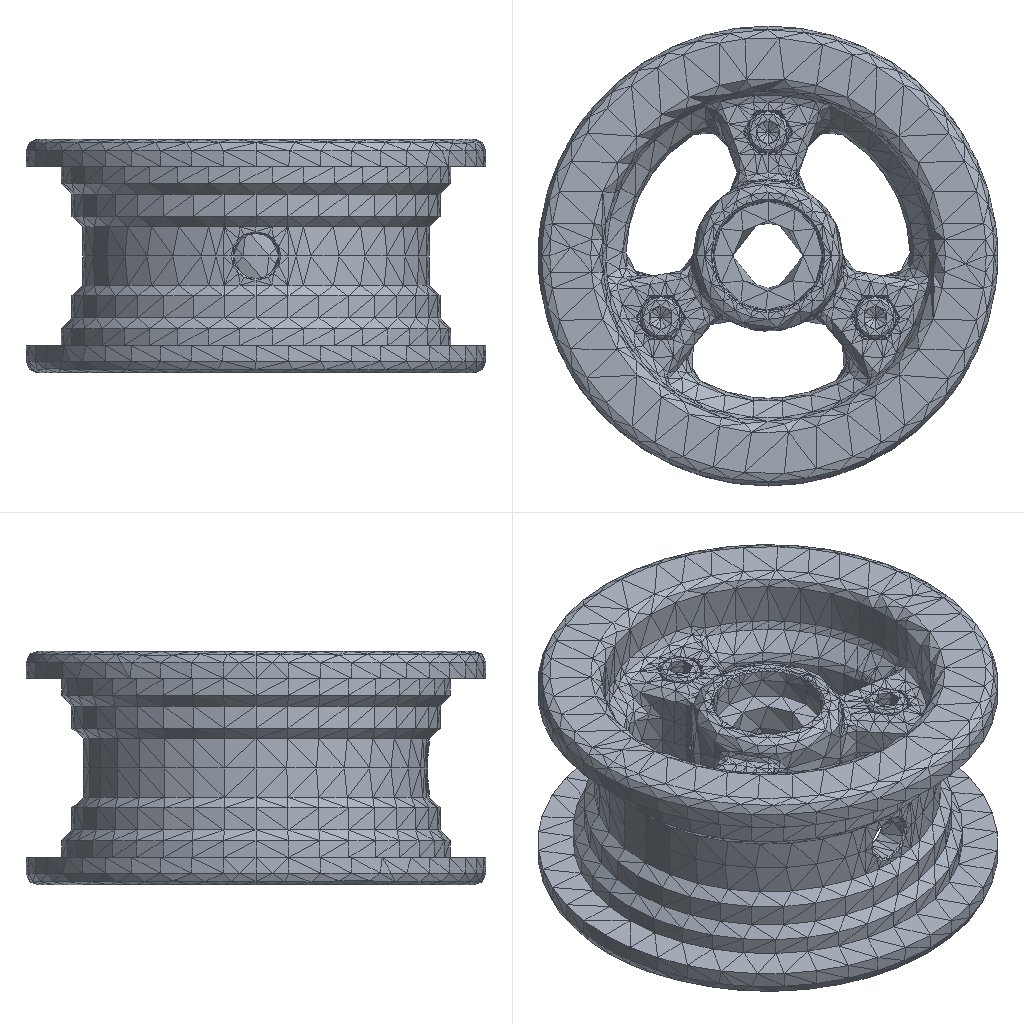Simulation study | ansys workbench
Ansys APDL input file, long lists of numbers shortened:
/batch
/config,noeldb,1     ! force off writing results to database
*get,_wallstrt,active,,time,wall
! ANSYS input file written by Workbench version 2022 R1
! File used for geometry attach:
/title,wbnew--__ (B5)
! ****** Begin Custom Load Command Snippet ******
/COM, ACT Extensions:
/COM,     LSDYNA, 2021.1
/COM,
! ****** End   Custom Load Command Snippet ******
*DIM,_wb_ProjectScratch_dir,string,248
_wb_ProjectScratch_dir(1) = ''
*DIM,_wb_SolverFiles_dir,string,248
_wb_SolverFiles_dir(1) = ''
*DIM,_wb_userfiles_dir,string,248
_wb_userfiles_dir(1) = ''
/com,--- Data in consistent NMM units. See Solving Units in the help system for more information.
/units,MPA
/nopr
/wb,file,start              !  signify a WB generated input file
/prep7
! Turn off shape checking because checks already performed inside WB mesher.
! See help system for more information.
SHPP,OFF,,NOWARN
/nolist
etcon,set             ! allow ANSYS to choose best KEYOP's for 180x elements, resets any applicable keyopt to MAPDL defaults
/com,*********** Nodes for the whole assembly ***********
nblock,3,,38121
(1i9,3e20.9e3)
        1    -7.914531287E+01    -4.780604649E+00     3.826096569E+01
! (34655 more lines like these left out)
-1
/wb,elem,start            !  set before creation of elements
/com,*********** Elements for Body 1 "Wheel Hub|Pah4" ***********
et,1,187
eblock,19,solid,,6596
(19i9)
        1        1        1        1        0        0        0        0       10        0     5341    10933    11707    12259    11913    16847    20987    16852    16849
! (13191 more lines like these left out)
-1
/com,*********** Elements for Body 2 "Wheel Hub|Pah4[2]" ***********
et,2,187
eblock,19,solid,,6596
(19i9)
        2        2        2        2        0        0        0        0       10        0    11937    23119    23893    24445    24099    29033    33173    29038    29035
! (13191 more lines like these left out)
-1
/com,*********** Elements for Body 3 "socket head cap screw_am32323_PreviewCfg|____1" ***********
et,3,187
eblock,19,solid,,671
(19i9)
        3        3        3        3        0        0        0        0       10        0     1343     2584     2701     2791     2775     2902     3548     2908     2906
! (1341 more lines like these left out)
-1
/com,*********** Elements for Body 4 "socket head cap screw_am32323_PreviewCfg|____1[2]" ***********
et,4,187
eblock,19,solid,,671
(19i9)
        4        4        4        4        0        0        0        0       10        0        1       12      129      219      203      330      976      336      334
! (1341 more lines like these left out)
-1
/com,*********** Elements for Body 5 "socket head cap screw_am32323_PreviewCfg|____1[3]" ***********
et,5,187
eblock,19,solid,,671
(19i9)
        5        5        5        5        0        0        0        0       10        0      672     1298     1415     1505     1489     1616     2262     1622     1620
! (1341 more lines like these left out)
-1
/com,*********** Elements for Body 6 "hex nut style 1_am333_PreviewCfg|____1" ***********
et,6,187
eblock,19,solid,,1109
(19i9)
        6        6        6        6        0        0        0        0       10        0     2014     4166     4227     4189     4221     5872     5956     5868     5870
! (2217 more lines like these left out)
-1
/com,*********** Elements for Body 7 "hex nut style 1_am333_PreviewCfg|____1[2]" ***********
et,7,187
eblock,19,solid,,1109
(19i9)
        7        7        7        7        0        0        0        0       10        0     3123     6308     6369     6331     6363     8014     8098     8010     8012
! (2217 more lines like these left out)
-1
/com,*********** Elements for Body 8 "hex nut style 1_am333_PreviewCfg|____1[3]" ***********
et,8,187
eblock,19,solid,,1109
(19i9)
        8        8        8        8        0        0        0        0       10        0     4232     8450     8511     8473     8505    10156    10240    10152    10154
! (2217 more lines like these left out)
-1
/wb,elem,end               !  done creating elements
/com,*********** Send User Defined Coordinate System(s) ***********
csys,0
toffst,273.15,  ! Temperature offset from absolute zero
/com,*********** Set Reference Temperature ***********
tref,22.
/wb,mat,start              !  starting to send materials
/com,*********** Send Materials ***********
Temperature = 'TEMP' ! Temperature
MP,DENS,1,7.85e-09,	! tonne mm^-3
MP,ALPX,1,1.2e-05,	! C^-1
MP,C,1,434000000,	! mm^2 s^-2 C^-1
MP,KXX,1,60.5,	! tonne mm s^-3 C^-1
MP,RSVX,1,0.00017,	! ohm mm
MP,EX,1,200000,	! tonne s^-2 mm^-1
MP,NUXY,1,0.3,
MP,MURX,1,10000,
Temperature = 'TEMP' ! Temperature
MP,DENS,2,7.85e-09,	! tonne mm^-3
MP,ALPX,2,1.2e-05,	! C^-1
MP,C,2,434000000,	! mm^2 s^-2 C^-1
MP,KXX,2,60.5,	! tonne mm s^-3 C^-1
MP,RSVX,2,0.00017,	! ohm mm
MP,EX,2,200000,	! tonne s^-2 mm^-1
MP,NUXY,2,0.3,
MP,MURX,2,10000,
Temperature = 'TEMP' ! Temperature
MP,DENS,3,7.85e-09,	! tonne mm^-3
MP,ALPX,3,1.2e-05,	! C^-1
MP,C,3,434000000,	! mm^2 s^-2 C^-1
MP,KXX,3,60.5,	! tonne mm s^-3 C^-1
MP,RSVX,3,0.00017,	! ohm mm
MP,EX,3,200000,	! tonne s^-2 mm^-1
MP,NUXY,3,0.3,
MP,MURX,3,10000,
Temperature = 'TEMP' ! Temperature
MP,DENS,4,7.85e-09,	! tonne mm^-3
MP,ALPX,4,1.2e-05,	! C^-1
MP,C,4,434000000,	! mm^2 s^-2 C^-1
MP,KXX,4,60.5,	! tonne mm s^-3 C^-1
MP,RSVX,4,0.00017,	! ohm mm
MP,EX,4,200000,	! tonne s^-2 mm^-1
MP,NUXY,4,0.3,
MP,MURX,4,10000,
Temperature = 'TEMP' ! Temperature
MP,DENS,5,7.85e-09,	! tonne mm^-3
MP,ALPX,5,1.2e-05,	! C^-1
MP,C,5,434000000,	! mm^2 s^-2 C^-1
MP,KXX,5,60.5,	! tonne mm s^-3 C^-1
MP,RSVX,5,0.00017,	! ohm mm
MP,EX,5,200000,	! tonne s^-2 mm^-1
MP,NUXY,5,0.3,
MP,MURX,5,10000,
Temperature = 'TEMP' ! Temperature
MP,DENS,6,7.85e-09,	! tonne mm^-3
MP,ALPX,6,1.2e-05,	! C^-1
MP,C,6,434000000,	! mm^2 s^-2 C^-1
MP,KXX,6,60.5,	! tonne mm s^-3 C^-1
MP,RSVX,6,0.00017,	! ohm mm
MP,EX,6,200000,	! tonne s^-2 mm^-1
MP,NUXY,6,0.3,
MP,MURX,6,10000,
Temperature = 'TEMP' ! Temperature
MP,DENS,7,7.85e-09,	! tonne mm^-3
MP,ALPX,7,1.2e-05,	! C^-1
MP,C,7,434000000,	! mm^2 s^-2 C^-1
MP,KXX,7,60.5,	! tonne mm s^-3 C^-1
MP,RSVX,7,0.00017,	! ohm mm
MP,EX,7,200000,	! tonne s^-2 mm^-1
MP,NUXY,7,0.3,
MP,MURX,7,10000,
Temperature = 'TEMP' ! Temperature
MP,DENS,8,7.85e-09,	! tonne mm^-3
MP,ALPX,8,1.2e-05,	! C^-1
MP,C,8,434000000,	! mm^2 s^-2 C^-1
MP,KXX,8,60.5,	! tonne mm s^-3 C^-1
MP,RSVX,8,0.00017,	! ohm mm
MP,EX,8,200000,	! tonne s^-2 mm^-1
MP,NUXY,8,0.3,
MP,MURX,8,10000,
/wb,mat,end                !  done sending materials
!************************* Model Summary ********************
!Wheel Hub|Pah4,	结构钢,	matid,	1
!Wheel Hub|Pah4[2],	结构钢,	matid,	2
!socket head cap screw_am32323_PreviewCfg|____1,	结构钢,	matid,	3
!socket head cap screw_am32323_PreviewCfg|____1[2],	结构钢,	matid,	4
!socket head cap screw_am32323_PreviewCfg|____1[3],	结构钢,	matid,	5
!hex nut style 1_am333_PreviewCfg|____1,	结构钢,	matid,	6
!hex nut style 1_am333_PreviewCfg|____1[2],	结构钢,	matid,	7
!hex nut style 1_am333_PreviewCfg|____1[3],	结构钢,	matid,	8
!************************* End Model Summary ********************
! get the diagonal of the bounding box. Needed later for other things
*get,_xmin,node,,mnloc,x
*get,_ymin,node,,mnloc,y
*get,_zmin,node,,mnloc,z
*get,_xmax,node,,mxloc,x
*get,_ymax,node,,mxloc,y
*get,_zmax,node,,mxloc,z
_ASMDIAG=(_xmax-_xmin)*(_xmax-_xmin)+(_ymax-_ymin)*(_ymax-_ymin)+(_zmax-_zmin)*(_zmax-_zmin)
_ASMDIAG=SQRT(_ASMDIAG)
/wb,contact,start          !  starting to send contact
/com,*********** Create Contact "接触区域" ***********
/com,            Real Constant Set For Above Contact Is 10 & 9
*set,tid,10
*set,cid,9
r,tid
r,cid
et,tid,170
et,cid,174
eblock,10,,,292
(15i9)
    27843       10       10       10        0    10309    10311    10313    10313    12419    12436    10313    12420
! (291 more lines like these left out)
-1
eblock,10,,,292
(15i9)
    28135        9        9        9        0    10309    10311    10313    10313    12419    12436    10313    12420
! (291 more lines like these left out)
-1
eblock,10,,,292
(15i9)
    28427        9       10        9        0    22510    22980    23548    23548    24717    28080    23548    24718
! (291 more lines like these left out)
-1
eblock,10,,,292
(15i9)
    28719       10        9       10        0    22510    22980    23548    23548    24717    28080    23548    24718
! (291 more lines like these left out)
-1
keyo,cid,8,2               ! auto create asymmetric contact (from Program Controlled setting)
keyo,cid,10,0              ! adjust contact stiffness each NR iteration (from Program Controlled setting)
keyo,cid,12,5              ! bonded always
keyo,cid,18,1              ! small sliding turned on by application
keyo,cid,2,0               ! augmented Lagrange (from Program Controlled setting)
keyo,cid,4,0               ! on Gauss point (from Program Controlled setting)
keyo,cid,9,1               ! ignore initial gaps/penetration
keyo,cid,7,0               ! No Prediction
rmod,tid,3,10.      ! FKN
rmod,tid,5,0.       ! ICONT
rmod,tid,6,0.       ! PINB
rmod,tid,10,0.      ! CNOF
rmod,tid,12,0.      ! FKT
rmod,tid,36,47      ! WB DSID
rmod,cid,3,10.      ! FKN
rmod,cid,5,0.       ! ICONT
rmod,cid,6,0.       ! PINB
rmod,cid,10,0.      ! CNOF
rmod,cid,12,0.      ! FKT
rmod,cid,36,47      ! WB DSID
/com,*********** Create Contact "接触区域 2" ***********
/com,            Real Constant Set For Above Contact Is 12 & 11
*set,tid,12
*set,cid,11
r,tid
r,cid
et,tid,170
et,cid,174
eblock,10,,,78
(15i9)
    29011       12       12       12        0    10732    10733    11268    11268    15538    15545    11268    15539
! (77 more lines like these left out)
-1
eblock,10,,,78
(15i9)
    29089       11       11       11        0    10732    10733    11268    11268    15538    15545    11268    15539
! (77 more lines like these left out)
-1
eblock,10,,,120
(15i9)
    29167       11       12       11        0     2686     2685     2589     2589     3470     2943     2589     2944
! (119 more lines like these left out)
-1
eblock,10,,,120
(15i9)
    29287       12       11       12        0     2686     2685     2589     2589     3470     2943     2589     2944
! (119 more lines like these left out)
-1
keyo,cid,8,2               ! auto create asymmetric contact (from Program Controlled setting)
keyo,cid,10,0              ! adjust contact stiffness each NR iteration (from Program Controlled setting)
keyo,cid,12,5              ! bonded always
keyo,cid,18,1              ! small sliding turned on by application
keyo,cid,2,0               ! augmented Lagrange (from Program Controlled setting)
keyo,cid,4,0               ! on Gauss point (from Program Controlled setting)
keyo,cid,9,1               ! ignore initial gaps/penetration
keyo,cid,7,0               ! No Prediction
rmod,tid,3,10.      ! FKN
rmod,tid,5,0.       ! ICONT
rmod,tid,6,0.       ! PINB
rmod,tid,10,0.      ! CNOF
rmod,tid,12,0.      ! FKT
rmod,tid,36,50      ! WB DSID
rmod,cid,3,10.      ! FKN
rmod,cid,5,0.       ! ICONT
rmod,cid,6,0.       ! PINB
rmod,cid,10,0.      ! CNOF
rmod,cid,12,0.      ! FKT
rmod,cid,36,50      ! WB DSID
/com,*********** Create Contact "接触区域 3" ***********
/com,            Real Constant Set For Above Contact Is 14 & 13
*set,tid,14
*set,cid,13
r,tid
r,cid
et,tid,170
et,cid,174
eblock,10,,,78
(15i9)
    29407       14       14       14        0    10740    11282    11277    11277    15595    19068    11277    15594
! (77 more lines like these left out)
-1
eblock,10,,,78
(15i9)
    29485       13       13       13        0    10740    11282    11277    11277    15595    19068    11277    15594
! (77 more lines like these left out)
-1
eblock,10,,,120
(15i9)
    29563       13       14       13        0      114      113       17       17      898      371       17      372
! (119 more lines like these left out)
-1
eblock,10,,,120
(15i9)
    29683       14       13       14        0      114      113       17       17      898      371       17      372
! (119 more lines like these left out)
-1
keyo,cid,8,2               ! auto create asymmetric contact (from Program Controlled setting)
keyo,cid,10,0              ! adjust contact stiffness each NR iteration (from Program Controlled setting)
keyo,cid,12,5              ! bonded always
keyo,cid,18,1              ! small sliding turned on by application
keyo,cid,2,0               ! augmented Lagrange (from Program Controlled setting)
keyo,cid,4,0               ! on Gauss point (from Program Controlled setting)
keyo,cid,9,1               ! ignore initial gaps/penetration
keyo,cid,7,0               ! No Prediction
rmod,tid,3,10.      ! FKN
rmod,tid,5,0.       ! ICONT
rmod,tid,6,0.       ! PINB
rmod,tid,10,0.      ! CNOF
rmod,tid,12,0.      ! FKT
rmod,tid,36,53      ! WB DSID
rmod,cid,3,10.      ! FKN
rmod,cid,5,0.       ! ICONT
rmod,cid,6,0.       ! PINB
rmod,cid,10,0.      ! CNOF
rmod,cid,12,0.      ! FKT
rmod,cid,36,53      ! WB DSID
/com,*********** Create Contact "接触区域 4" ***********
/com,            Real Constant Set For Above Contact Is 16 & 15
*set,tid,16
*set,cid,15
r,tid
r,cid
et,tid,170
et,cid,174
eblock,10,,,96
(15i9)
    29803       16       16       16        0    10722    11519    10954    10954    15475    17014    10954    15472
! (95 more lines like these left out)
-1
eblock,10,,,96
(15i9)
    29899       15       15       15        0    10722    11519    10954    10954    15475    17014    10954    15472
! (95 more lines like these left out)
-1
eblock,10,,,120
(15i9)
    29995       15       16       15        0     1400     1399     1303     1303     2184     1657     1303     1658
! (119 more lines like these left out)
-1
eblock,10,,,120
(15i9)
    30115       16       15       16        0     1400     1399     1303     1303     2184     1657     1303     1658
! (119 more lines like these left out)
-1
keyo,cid,8,2               ! auto create asymmetric contact (from Program Controlled setting)
keyo,cid,10,0              ! adjust contact stiffness each NR iteration (from Program Controlled setting)
keyo,cid,12,5              ! bonded always
keyo,cid,18,1              ! small sliding turned on by application
keyo,cid,2,0               ! augmented Lagrange (from Program Controlled setting)
keyo,cid,4,0               ! on Gauss point (from Program Controlled setting)
keyo,cid,9,1               ! ignore initial gaps/penetration
keyo,cid,7,0               ! No Prediction
rmod,tid,3,10.      ! FKN
rmod,tid,5,0.       ! ICONT
rmod,tid,6,0.       ! PINB
rmod,tid,10,0.      ! CNOF
rmod,tid,12,0.      ! FKT
rmod,tid,36,56      ! WB DSID
rmod,cid,3,10.      ! FKN
rmod,cid,5,0.       ! ICONT
rmod,cid,6,0.       ! PINB
rmod,cid,10,0.      ! CNOF
rmod,cid,12,0.      ! FKT
rmod,cid,36,56      ! WB DSID
/com,*********** Create Contact "接触区域 5" ***********
/com,            Real Constant Set For Above Contact Is 18 & 17
*set,tid,18
*set,cid,17
r,tid
r,cid
et,tid,170
et,cid,174
eblock,10,,,12
(15i9)
    30235       18       18       18        0    22918    22919    23454    23454    27724    27731    23454    27725
! (11 more lines like these left out)
-1
eblock,10,,,12
(15i9)
    30247       17       17       17        0    22918    22919    23454    23454    27724    27731    23454    27725
! (11 more lines like these left out)
-1
eblock,10,,,154
(15i9)
    30259       17       18       17        0     4023     4081     4131     4131     5259     5447     4131     5261
! (153 more lines like these left out)
-1
eblock,10,,,154
(15i9)
    30413       18       17       18        0     4023     4081     4131     4131     5259     5447     4131     5261
! (153 more lines like these left out)
-1
keyo,cid,8,2               ! auto create asymmetric contact (from Program Controlled setting)
keyo,cid,10,0              ! adjust contact stiffness each NR iteration (from Program Controlled setting)
keyo,cid,12,5              ! bonded always
keyo,cid,18,1              ! small sliding turned on by application
keyo,cid,2,0               ! augmented Lagrange (from Program Controlled setting)
keyo,cid,4,0               ! on Gauss point (from Program Controlled setting)
keyo,cid,9,1               ! ignore initial gaps/penetration
keyo,cid,7,0               ! No Prediction
rmod,tid,3,10.      ! FKN
rmod,tid,5,0.       ! ICONT
rmod,tid,6,0.       ! PINB
rmod,tid,10,0.      ! CNOF
rmod,tid,12,0.      ! FKT
rmod,tid,36,59      ! WB DSID
rmod,cid,3,10.      ! FKN
rmod,cid,5,0.       ! ICONT
rmod,cid,6,0.       ! PINB
rmod,cid,10,0.      ! CNOF
rmod,cid,12,0.      ! FKT
rmod,cid,36,59      ! WB DSID
/com,*********** Create Contact "接触区域 6" ***********
/com,            Real Constant Set For Above Contact Is 20 & 19
*set,tid,20
*set,cid,19
r,tid
r,cid
et,tid,170
et,cid,174
eblock,10,,,19
(15i9)
    30567       20       20       20        0    22908    23705    23140    23140    27661    29200    23140    27658
! (18 more lines like these left out)
-1
eblock,10,,,19
(15i9)
    30586       19       19       19        0    22908    23705    23140    23140    27661    29200    23140    27658
! (18 more lines like these left out)
-1
eblock,10,,,147
(15i9)
    30605       19       20       19        0     6165     6223     6273     6273     7401     7589     6273     7403
! (146 more lines like these left out)
-1
eblock,10,,,147
(15i9)
    30752       20       19       20        0     6165     6223     6273     6273     7401     7589     6273     7403
! (146 more lines like these left out)
-1
keyo,cid,8,2               ! auto create asymmetric contact (from Program Controlled setting)
keyo,cid,10,0              ! adjust contact stiffness each NR iteration (from Program Controlled setting)
keyo,cid,12,5              ! bonded always
keyo,cid,18,1              ! small sliding turned on by application
keyo,cid,2,0               ! augmented Lagrange (from Program Controlled setting)
keyo,cid,4,0               ! on Gauss point (from Program Controlled setting)
keyo,cid,9,1               ! ignore initial gaps/penetration
keyo,cid,7,0               ! No Prediction
rmod,tid,3,10.      ! FKN
rmod,tid,5,0.       ! ICONT
rmod,tid,6,0.       ! PINB
rmod,tid,10,0.      ! CNOF
rmod,tid,12,0.      ! FKT
rmod,tid,36,62      ! WB DSID
rmod,cid,3,10.      ! FKN
rmod,cid,5,0.       ! ICONT
rmod,cid,6,0.       ! PINB
rmod,cid,10,0.      ! CNOF
rmod,cid,12,0.      ! FKT
rmod,cid,36,62      ! WB DSID
/com,*********** Create Contact "接触区域 7" ***********
/com,            Real Constant Set For Above Contact Is 22 & 21
*set,tid,22
*set,cid,21
r,tid
r,cid
et,tid,170
et,cid,174
eblock,10,,,12
(15i9)
    30899       22       22       22        0    22926    23468    23463    23463    27781    31254    23463    27780
! (11 more lines like these left out)
-1
eblock,10,,,12
(15i9)
    30911       21       21       21        0    22926    23468    23463    23463    27781    31254    23463    27780
! (11 more lines like these left out)
-1
eblock,10,,,154
(15i9)
    30923       21       22       21        0     8307     8365     8415     8415     9543     9731     8415     9545
! (153 more lines like these left out)
-1
eblock,10,,,154
(15i9)
    31077       22       21       22        0     8307     8365     8415     8415     9543     9731     8415     9545
! (153 more lines like these left out)
-1
keyo,cid,8,2               ! auto create asymmetric contact (from Program Controlled setting)
keyo,cid,10,0              ! adjust contact stiffness each NR iteration (from Program Controlled setting)
keyo,cid,12,5              ! bonded always
keyo,cid,18,1              ! small sliding turned on by application
keyo,cid,2,0               ! augmented Lagrange (from Program Controlled setting)
keyo,cid,4,0               ! on Gauss point (from Program Controlled setting)
keyo,cid,9,1               ! ignore initial gaps/penetration
keyo,cid,7,0               ! No Prediction
rmod,tid,3,10.      ! FKN
rmod,tid,5,0.       ! ICONT
rmod,tid,6,0.       ! PINB
rmod,tid,10,0.      ! CNOF
rmod,tid,12,0.      ! FKT
rmod,tid,36,65      ! WB DSID
rmod,cid,3,10.      ! FKN
rmod,cid,5,0.       ! ICONT
rmod,cid,6,0.       ! PINB
rmod,cid,10,0.      ! CNOF
rmod,cid,12,0.      ! FKT
rmod,cid,36,65      ! WB DSID
nsel,all
esel,all
/wb,contact,end            !  done creating contacts
/golist
/wb,load,start             !  starting to send loads
/gst,on,on
fini
*get,_numnode,node,0,count
*get,_numelem,elem,0,count
*get, _MAXELEMNUM, elem, 0, NUM, MAX
*get, _MAXNODENUM, node, 0, NUM, MAX
*get, _MAXELEMTYPE, etyp, 0, NUM, MAX
*get, _MAXREALCONST, real, 0, NUM, MAX
/go
/wb,load,end               !  done creating loads
/com,--- Number of total nodes = %_numnode%
/com,--- Number of contact elements = 3388
/com,--- Number of spring elements = 0
/com,--- Number of bearing elements = 0
/com,--- Number of solid elements = 18532
/com,--- Number of condensed parts = 0
/com,--- Number of total elements = %_numelem%
*get,_wallbsol,active,,time,wall
/solu
antype,2                   ! modal analysis
_thickRatio=  1     ! Ratio of thick parts in the model
modopt,lanb,6
outres,erase
outres,all,none
outres,nsol,all
outres,etmp,all
mxpand                    ! default expand in case of complex solution
dmpopt,esav,no
dmpopt,emat,no
dmpopt,full,no
! *********** WB SOLVE COMMAND ***********
! check interactive state
*get,ANSINTER_,active,,int
*if,ANSINTER_,ne,0,then
/eof
*endif
solve
/com *************** Write FE CONNECTORS *********
CEWRITE,file,ce,,INTE
*get,_nmodalsolproc,active,0,numcpu
fini
/nopr
*get,_numnode,node,0,count
*get,_numelem,elem,0,count
*get, _MAXELEMNUM, elem, 0, NUM, MAX
*get, _MAXNODENUM, node, 0, NUM, MAX,,,INTERNAL
*get, _MAXELEMTYPE, etyp, 0, NUM, MAX
*get, _MAXREALCONST, real, 0, NUM, MAX
/gopr
*get,_wallasol,active,,time,wall
/post1
/nopr
*dim,_direction,CHAR,6,1
_direction(1) = 'X'
_direction(2) = 'Y'
_direction(3) = 'Z'
_direction(4) = 'ROTX'
_direction(5) = 'ROTY'
_direction(6) = 'ROTZ'
*get,_lastLS,active,0,set,LSTP
*get,_beginset,active,0,set,nset,first,_lastLS
*get,_endset,active,0,set,nset,last,_lastLS
_nummodes = 0
*if,_endset,gt,0,then
_nummodes = _endset - _beginset + 1
*endif
*do,i_mode,1,_nummodes
   *do,j_component,1,6
			*get,PFACT_%i_mode%_%j_component%,MODE,%i_mode%,PFACT,,DIREC,_direction(%j_component%)
   *enddo
*enddo
*dim,_tmdirection,CHAR,6,1
_tmdirection(1) = 'X'
_tmdirection(2) = 'Y'
_tmdirection(3) = 'Z'
_tmdirection(4) = 'X'
_tmdirection(5) = 'Y'
_tmdirection(6) = 'Z'
*do,j_component,1,6
    *if,j_component,gt,3,then
        *get,TOTALMASS_%j_component%,ELEM,0,IOR,_tmdirection(%j_component%)
    *else
        *get,TOTALMASS_%j_component%,ELEM,0,MTOT,_tmdirection(%j_component%)
    *endif
*enddo
/gopr
xmlo,ENCODING,ISO-8859-1
xmlo,parm
/xml,parm,xml
fini
/gopr
*get,_walldone,active,,time,wall
_preptime=(_wallbsol-_wallstrt)*3600
_solvtime=(_wallasol-_wallbsol)*3600
_posttime=(_walldone-_wallasol)*3600
_totaltim=(_walldone-_wallstrt)*3600
*get,_dlbratio,active,0,solu,dlbr
*get,_combtime,active,0,solu,comb
*get,_ssmode,active,0,solu,ssmm
*get,_ndofs,active,0,solu,ndof
/fclean				!clean distributed files
/com,--- Total number of nodes = %_numnode%
/com,--- Total number of elements = %_numelem%
/com,--- Element load balance ratio = %_dlbratio%
/com,--- Time to combine distributed files = %_combtime%
/com,--- Sparse memory mode = %_ssmode%
/com,--- Number of DOF = %_ndofs%
/wb,file,end               ! done with WB generated input